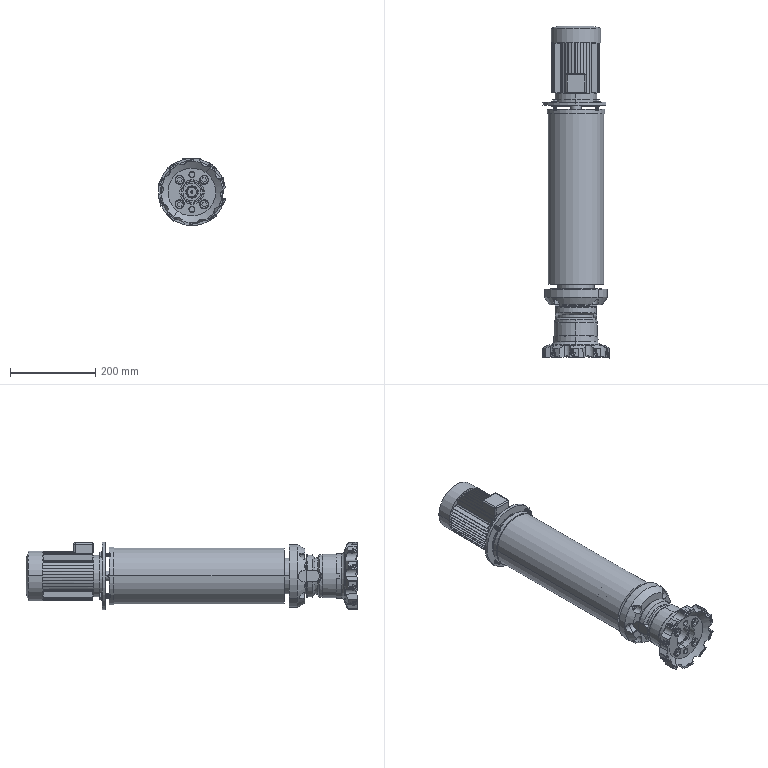Part | SolidWorks | 163 solids | 3809 faces | volume 7727632 mm3 | plane 1169 | cone 887 | cylinder 796 | torus 733 | sphere 204 | spline 20 | commonest cylinder face diameters 8 x163 4.8 x46 97.2 x40 165.792 x40 7.92 x39 4 x27